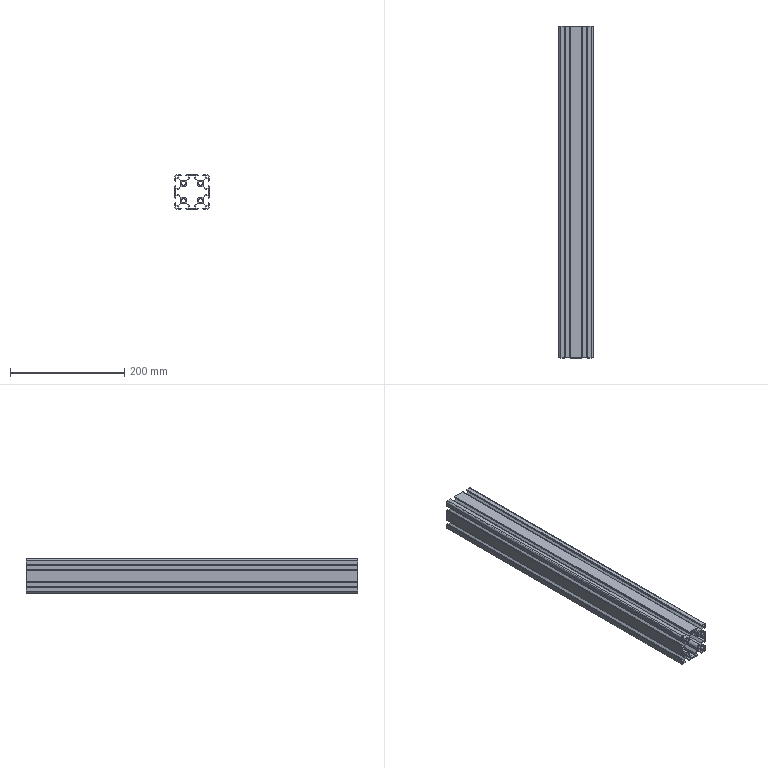Part | STEP file | PN_0025 Lower outer frame column_Default <Machined> | 1 solid | 178 faces | box 60 x 580 x 60 mm | volume 533826 mm3 | plane 162 | cylinder 16 | commonest cylinder face diameters 6.8 x8 6.76 x4 11.828 x4